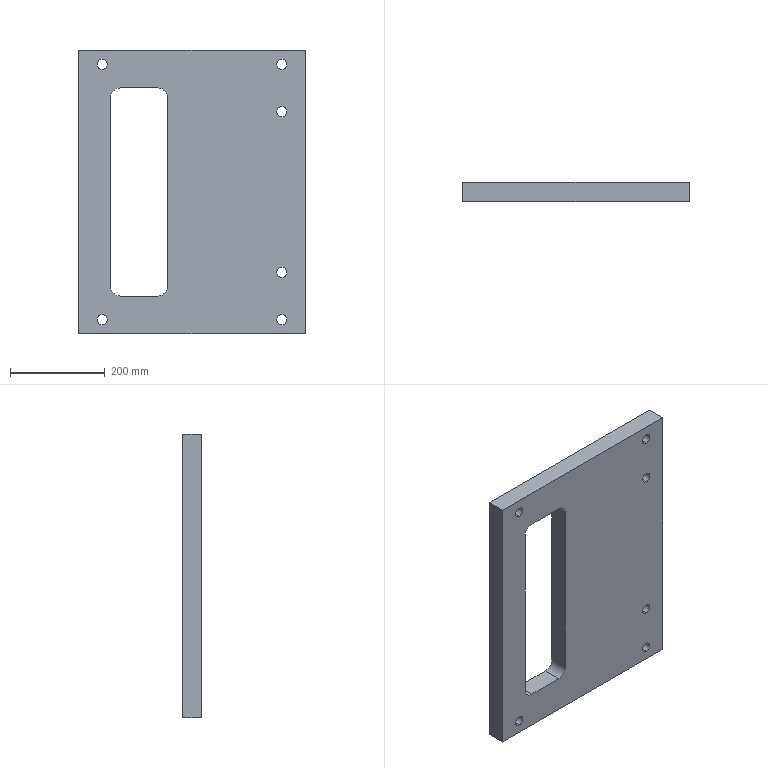Part | SolidWorks | features Extrusion 1, Fillet 1, HoleWzd 1, ICE 1 | 1 solid | 26 faces | box 480 x 40 x 600 mm | volume 9338608 mm3 | cylinder 16 | plane 10 | commonest cylinder face diameters 21 x12 40 x4
STEP:
#1=CARTESIAN_POINT('',(-190.,0.,259.5));
#2=VERTEX_POINT('',#1);
#3=CARTESIAN_POINT('',(-190.,0.,280.5));
#4=VERTEX_POINT('',#3);
#5=CARTESIAN_POINT('',(-190.,0.,270.));
#6=DIRECTION('',(0.,1.,0.));
#7=DIRECTION('',(0.,0.,1.));
#8=AXIS2_PLACEMENT_3D('',#5,#6,#7);
#9=CIRCLE('',#8,10.5);
#10=EDGE_CURVE('',#2,#4,#9,.T.);
#11=ORIENTED_EDGE('',*,*,#10,.F.);
#12=CARTESIAN_POINT('',(-190.,40.,259.5));
#13=VERTEX_POINT('',#12);
#14=CARTESIAN_POINT('',(-190.,40.,259.5));
#15=DIRECTION('',(0.,1.,0.));
#16=VECTOR('',#15,1000.);
#17=LINE('',#14,#16);
#18=EDGE_CURVE('',#2,#13,#17,.T.);
#19=ORIENTED_EDGE('',*,*,#18,.T.);
#20=CARTESIAN_POINT('',(-190.,40.,280.5));
#21=VERTEX_POINT('',#20);
#22=CARTESIAN_POINT('',(-190.,40.,270.));
#23=DIRECTION('',(0.,1.,0.));
#24=DIRECTION('',(0.,0.,1.));
#25=AXIS2_PLACEMENT_3D('',#22,#23,#24);
#26=CIRCLE('',#25,10.5);
#27=EDGE_CURVE('',#13,#21,#26,.T.);
#28=ORIENTED_EDGE('',*,*,#27,.T.);
#29=CARTESIAN_POINT('',(-190.,40.,280.5));
#30=DIRECTION('',(0.,1.,0.));
#31=VECTOR('',#30,1000.);
#32=LINE('',#29,#31);
#33=EDGE_CURVE('',#4,#21,#32,.T.);
#34=ORIENTED_EDGE('',*,*,#33,.F.);
#35=EDGE_LOOP('',(#11,#19,#28,#34));
#36=FACE_OUTER_BOUND('',#35,.T.);
#37=CARTESIAN_POINT('',(-190.,40.,270.));
#38=DIRECTION('',(0.,1.,0.));
#39=DIRECTION('',(0.,0.,1.));
#40=AXIS2_PLACEMENT_3D('',#37,#38,#39);
#41=CYLINDRICAL_SURFACE('',#40,10.5);
#42=ADVANCED_FACE('',(#36),#41,.F.);
#43=CARTESIAN_POINT('',(-190.,0.,-280.5));
#44=VERTEX_POINT('',#43);
#45=CARTESIAN_POINT('',(-190.,0.,-259.5));
#46=VERTEX_POINT('',#45);
#47=CARTESIAN_POINT('',(-190.,0.,-270.));
#48=DIRECTION('',(0.,1.,0.));
#49=DIRECTION('',(0.,0.,1.));
#50=AXIS2_PLACEMENT_3D('',#47,#48,#49);
#51=CIRCLE('',#50,10.5);
#52=EDGE_CURVE('',#44,#46,#51,.T.);
#53=ORIENTED_EDGE('',*,*,#52,.F.);
#54=CARTESIAN_POINT('',(-190.,40.,-280.5));
#55=VERTEX_POINT('',#54);
#56=CARTESIAN_POINT('',(-190.,40.,-280.5));
#57=DIRECTION('',(0.,1.,0.));
#58=VECTOR('',#57,1000.);
#59=LINE('',#56,#58);
#60=EDGE_CURVE('',#44,#55,#59,.T.);
#61=ORIENTED_EDGE('',*,*,#60,.T.);
#62=CARTESIAN_POINT('',(-190.,40.,-259.5));
#63=VERTEX_POINT('',#62);
#64=CARTESIAN_POINT('',(-190.,40.,-270.));
#65=DIRECTION('',(0.,1.,0.));
#66=DIRECTION('',(0.,0.,1.));
#67=AXIS2_PLACEMENT_3D('',#64,#65,#66);
#68=CIRCLE('',#67,10.5);
#69=EDGE_CURVE('',#55,#63,#68,.T.);
#70=ORIENTED_EDGE('',*,*,#69,.T.);
#71=CARTESIAN_POINT('',(-190.,40.,-259.5));
#72=DIRECTION('',(0.,1.,0.));
#73=VECTOR('',#72,1000.);
#74=LINE('',#71,#73);
#75=EDGE_CURVE('',#46,#63,#74,.T.);
#76=ORIENTED_EDGE('',*,*,#75,.F.);
#77=EDGE_LOOP('',(#53,#61,#70,#76));
#78=FACE_OUTER_BOUND('',#77,.T.);
#79=CARTESIAN_POINT('',(-190.,40.,-270.));
#80=DIRECTION('',(0.,1.,0.));
#81=DIRECTION('',(0.,0.,1.));
#82=AXIS2_PLACEMENT_3D('',#79,#80,#81);
#83=CYLINDRICAL_SURFACE('',#82,10.5);
#84=ADVANCED_FACE('',(#78),#83,.F.);
#85=CARTESIAN_POINT('',(190.,0.,-280.5));
#86=VERTEX_POINT('',#85);
#87=CARTESIAN_POINT('',(190.,0.,-259.5));
#88=VERTEX_POINT('',#87);
#89=CARTESIAN_POINT('',(190.,0.,-270.));
#90=DIRECTION('',(0.,1.,0.));
#91=DIRECTION('',(0.,0.,1.));
#92=AXIS2_PLACEMENT_3D('',#89,#90,#91);
#93=CIRCLE('',#92,10.5);
#94=EDGE_CURVE('',#86,#88,#93,.T.);
#95=ORIENTED_EDGE('',*,*,#94,.F.);
#96=CARTESIAN_POINT('',(190.,40.,-280.5));
#97=VERTEX_POINT('',#96);
#98=CARTESIAN_POINT('',(190.,40.,-280.5));
#99=DIRECTION('',(0.,1.,0.));
#100=VECTOR('',#99,1000.);
#101=LINE('',#98,#100);
#102=EDGE_CURVE('',#86,#97,#101,.T.);
#103=ORIENTED_EDGE('',*,*,#102,.T.);
#104=CARTESIAN_POINT('',(190.,40.,-259.5));
#105=VERTEX_POINT('',#104);
#106=CARTESIAN_POINT('',(190.,40.,-270.));
#107=DIRECTION('',(0.,1.,0.));
#108=DIRECTION('',(0.,0.,1.));
#109=AXIS2_PLACEMENT_3D('',#106,#107,#108);
#110=CIRCLE('',#109,10.5);
#111=EDGE_CURVE('',#97,#105,#110,.T.);
#112=ORIENTED_EDGE('',*,*,#111,.T.);
#113=CARTESIAN_POINT('',(190.,40.,-259.5));
#114=DIRECTION('',(0.,1.,0.));
#115=VECTOR('',#114,1000.);
#116=LINE('',#113,#115);
#117=EDGE_CURVE('',#88,#105,#116,.T.);
#118=ORIENTED_EDGE('',*,*,#117,.F.);
#119=EDGE_LOOP('',(#95,#103,#112,#118));
#120=FACE_OUTER_BOUND('',#119,.T.);
#121=CARTESIAN_POINT('',(190.,40.,-270.));
#122=DIRECTION('',(0.,1.,0.));
#123=DIRECTION('',(0.,0.,1.));
#124=AXIS2_PLACEMENT_3D('',#121,#122,#123);
#125=CYLINDRICAL_SURFACE('',#124,10.5);
#126=ADVANCED_FACE('',(#120),#125,.F.);
#127=CARTESIAN_POINT('',(190.,0.,259.5));
#128=VERTEX_POINT('',#127);
#129=CARTESIAN_POINT('',(190.,0.,280.5));
#130=VERTEX_POINT('',#129);
#131=CARTESIAN_POINT('',(190.,0.,270.));
#132=DIRECTION('',(0.,1.,0.));
#133=DIRECTION('',(0.,0.,1.));
#134=AXIS2_PLACEMENT_3D('',#131,#132,#133);
#135=CIRCLE('',#134,10.5);
#136=EDGE_CURVE('',#128,#130,#135,.T.);
#137=ORIENTED_EDGE('',*,*,#136,.F.);
#138=CARTESIAN_POINT('',(190.,40.,259.5));
#139=VERTEX_POINT('',#138);
#140=CARTESIAN_POINT('',(190.,40.,259.5));
#141=DIRECTION('',(0.,1.,0.));
#142=VECTOR('',#141,1000.);
#143=LINE('',#140,#142);
#144=EDGE_CURVE('',#128,#139,#143,.T.);
#145=ORIENTED_EDGE('',*,*,#144,.T.);
#146=CARTESIAN_POINT('',(190.,40.,280.5));
#147=VERTEX_POINT('',#146);
#148=CARTESIAN_POINT('',(190.,40.,270.));
#149=DIRECTION('',(0.,1.,0.));
#150=DIRECTION('',(0.,0.,1.));
#151=AXIS2_PLACEMENT_3D('',#148,#149,#150);
#152=CIRCLE('',#151,10.5);
#153=EDGE_CURVE('',#139,#147,#152,.T.);
#154=ORIENTED_EDGE('',*,*,#153,.T.);
#155=CARTESIAN_POINT('',(190.,40.,280.5));
#156=DIRECTION('',(0.,1.,0.));
#157=VECTOR('',#156,1000.);
#158=LINE('',#155,#157);
#159=EDGE_CURVE('',#130,#147,#158,.T.);
#160=ORIENTED_EDGE('',*,*,#159,.F.);
#161=EDGE_LOOP('',(#137,#145,#154,#160));
#162=FACE_OUTER_BOUND('',#161,.T.);
#163=CARTESIAN_POINT('',(190.,40.,270.));
#164=DIRECTION('',(0.,1.,0.));
#165=DIRECTION('',(0.,0.,1.));
#166=AXIS2_PLACEMENT_3D('',#163,#164,#165);
#167=CYLINDRICAL_SURFACE('',#166,10.5);
#168=ADVANCED_FACE('',(#162),#167,.F.);
#169=CARTESIAN_POINT('',(190.,0.,-180.5));
#170=VERTEX_POINT('',#169);
#171=CARTESIAN_POINT('',(190.,0.,-159.5));
#172=VERTEX_POINT('',#171);
#173=CARTESIAN_POINT('',(190.,0.,-170.));
#174=DIRECTION('',(0.,1.,0.));
#175=DIRECTION('',(0.,0.,1.));
#176=AXIS2_PLACEMENT_3D('',#173,#174,#175);
#177=CIRCLE('',#176,10.5);
#178=EDGE_CURVE('',#170,#172,#177,.T.);
#179=ORIENTED_EDGE('',*,*,#178,.F.);
#180=CARTESIAN_POINT('',(190.,40.,-180.5));
#181=VERTEX_POINT('',#180);
#182=CARTESIAN_POINT('',(190.,40.,-180.5));
#183=DIRECTION('',(0.,1.,0.));
#184=VECTOR('',#183,1000.);
#185=LINE('',#182,#184);
#186=EDGE_CURVE('',#170,#181,#185,.T.);
#187=ORIENTED_EDGE('',*,*,#186,.T.);
#188=CARTESIAN_POINT('',(190.,40.,-159.5));
#189=VERTEX_POINT('',#188);
#190=CARTESIAN_POINT('',(190.,40.,-170.));
#191=DIRECTION('',(0.,1.,0.));
#192=DIRECTION('',(0.,0.,1.));
#193=AXIS2_PLACEMENT_3D('',#190,#191,#192);
#194=CIRCLE('',#193,10.5);
#195=EDGE_CURVE('',#181,#189,#194,.T.);
#196=ORIENTED_EDGE('',*,*,#195,.T.);
#197=CARTESIAN_POINT('',(190.,40.,-159.5));
#198=DIRECTION('',(0.,1.,0.));
#199=VECTOR('',#198,1000.);
#200=LINE('',#197,#199);
#201=EDGE_CURVE('',#172,#189,#200,.T.);
#202=ORIENTED_EDGE('',*,*,#201,.F.);
#203=EDGE_LOOP('',(#179,#187,#196,#202));
#204=FACE_OUTER_BOUND('',#203,.T.);
#205=CARTESIAN_POINT('',(190.,40.,-170.));
#206=DIRECTION('',(0.,1.,0.));
#207=DIRECTION('',(0.,0.,1.));
#208=AXIS2_PLACEMENT_3D('',#205,#206,#207);
#209=CYLINDRICAL_SURFACE('',#208,10.5);
#210=ADVANCED_FACE('',(#204),#209,.F.);
#211=CARTESIAN_POINT('',(190.,0.,159.5));
#212=VERTEX_POINT('',#211);
#213=CARTESIAN_POINT('',(190.,0.,180.5));
#214=VERTEX_POINT('',#213);
#215=CARTESIAN_POINT('',(190.,0.,170.));
#216=DIRECTION('',(0.,1.,0.));
#217=DIRECTION('',(0.,0.,1.));
#218=AXIS2_PLACEMENT_3D('',#215,#216,#217);
#219=CIRCLE('',#218,10.5);
#220=EDGE_CURVE('',#212,#214,#219,.T.);
#221=ORIENTED_EDGE('',*,*,#220,.F.);
#222=CARTESIAN_POINT('',(190.,40.,159.5));
#223=VERTEX_POINT('',#222);
#224=CARTESIAN_POINT('',(190.,40.,159.5));
#225=DIRECTION('',(0.,1.,0.));
#226=VECTOR('',#225,1000.);
#227=LINE('',#224,#226);
#228=EDGE_CURVE('',#212,#223,#227,.T.);
#229=ORIENTED_EDGE('',*,*,#228,.T.);
#230=CARTESIAN_POINT('',(190.,40.,180.5));
#231=VERTEX_POINT('',#230);
#232=CARTESIAN_POINT('',(190.,40.,170.));
#233=DIRECTION('',(0.,1.,0.));
#234=DIRECTION('',(0.,0.,1.));
#235=AXIS2_PLACEMENT_3D('',#232,#233,#234);
#236=CIRCLE('',#235,10.5);
#237=EDGE_CURVE('',#223,#231,#236,.T.);
#238=ORIENTED_EDGE('',*,*,#237,.T.);
#239=CARTESIAN_POINT('',(190.,40.,180.5));
#240=DIRECTION('',(0.,1.,0.));
#241=VECTOR('',#240,1000.);
#242=LINE('',#239,#241);
#243=EDGE_CURVE('',#214,#231,#242,.T.);
#244=ORIENTED_EDGE('',*,*,#243,.F.);
#245=EDGE_LOOP('',(#221,#229,#238,#244));
#246=FACE_OUTER_BOUND('',#245,.T.);
#247=CARTESIAN_POINT('',(190.,40.,170.));
#248=DIRECTION('',(0.,1.,0.));
#249=DIRECTION('',(0.,0.,1.));
#250=AXIS2_PLACEMENT_3D('',#247,#248,#249);
#251=CYLINDRICAL_SURFACE('',#250,10.5);
#252=ADVANCED_FACE('',(#246),#251,.F.);
#253=CARTESIAN_POINT('',(240.,0.,300.));
#254=VERTEX_POINT('',#253);
#255=CARTESIAN_POINT('',(240.,0.,-300.));
#256=VERTEX_POINT('',#255);
#257=CARTESIAN_POINT('',(240.,0.,-300.));
#258=DIRECTION('',(0.,0.,-1.));
#259=VECTOR('',#258,1000.);
#260=LINE('',#257,#259);
#261=EDGE_CURVE('',#254,#256,#260,.T.);
#262=ORIENTED_EDGE('',*,*,#261,.T.);
#263=CARTESIAN_POINT('',(240.,40.,-300.));
#264=VERTEX_POINT('',#263);
#265=CARTESIAN_POINT('',(240.,40.,-300.));
#266=DIRECTION('',(0.,-1.,0.));
#267=VECTOR('',#266,1000.);
#268=LINE('',#265,#267);
#269=EDGE_CURVE('',#264,#256,#268,.T.);
#270=ORIENTED_EDGE('',*,*,#269,.F.);
#271=CARTESIAN_POINT('',(240.,40.,300.));
#272=VERTEX_POINT('',#271);
#273=CARTESIAN_POINT('',(240.,40.,-300.));
#274=DIRECTION('',(0.,0.,-1.));
#275=VECTOR('',#274,1000.);
#276=LINE('',#273,#275);
#277=EDGE_CURVE('',#272,#264,#276,.T.);
#278=ORIENTED_EDGE('',*,*,#277,.F.);
#279=CARTESIAN_POINT('',(240.,40.,300.));
#280=DIRECTION('',(0.,-1.,0.));
#281=VECTOR('',#280,1000.);
#282=LINE('',#279,#281);
#283=EDGE_CURVE('',#272,#254,#282,.T.);
#284=ORIENTED_EDGE('',*,*,#283,.T.);
#285=EDGE_LOOP('',(#262,#270,#278,#284));
#286=FACE_OUTER_BOUND('',#285,.T.);
#287=CARTESIAN_POINT('',(240.,40.,-300.));
#288=DIRECTION('',(-1.,0.,0.));
#289=DIRECTION('',(0.,0.,1.));
#290=AXIS2_PLACEMENT_3D('',#287,#288,#289);
#291=PLANE('',#290);
#292=ADVANCED_FACE('',(#286),#291,.F.);
#293=CARTESIAN_POINT('',(-240.,0.,-300.));
#294=VERTEX_POINT('',#293);
#295=CARTESIAN_POINT('',(-240.,0.,-300.));
#296=DIRECTION('',(-1.,0.,0.));
#297=VECTOR('',#296,1000.);
#298=LINE('',#295,#297);
#299=EDGE_CURVE('',#256,#294,#298,.T.);
#300=ORIENTED_EDGE('',*,*,#299,.T.);
#301=CARTESIAN_POINT('',(-240.,40.,-300.));
#302=VERTEX_POINT('',#301);
#303=CARTESIAN_POINT('',(-240.,40.,-300.));
#304=DIRECTION('',(0.,-1.,0.));
#305=VECTOR('',#304,1000.);
#306=LINE('',#303,#305);
#307=EDGE_CURVE('',#302,#294,#306,.T.);
#308=ORIENTED_EDGE('',*,*,#307,.F.);
#309=CARTESIAN_POINT('',(-240.,40.,-300.));
#310=DIRECTION('',(-1.,0.,0.));
#311=VECTOR('',#310,1000.);
#312=LINE('',#309,#311);
#313=EDGE_CURVE('',#264,#302,#312,.T.);
#314=ORIENTED_EDGE('',*,*,#313,.F.);
#315=ORIENTED_EDGE('',*,*,#269,.T.);
#316=EDGE_LOOP('',(#300,#308,#314,#315));
#317=FACE_OUTER_BOUND('',#316,.T.);
#318=CARTESIAN_POINT('',(-240.,40.,-300.));
#319=DIRECTION('',(0.,0.,1.));
#320=DIRECTION('',(1.,0.,0.));
#321=AXIS2_PLACEMENT_3D('',#318,#319,#320);
#322=PLANE('',#321);
#323=ADVANCED_FACE('',(#317),#322,.F.);
#324=CARTESIAN_POINT('',(-240.,0.,300.));
#325=VERTEX_POINT('',#324);
#326=CARTESIAN_POINT('',(-240.,0.,-300.));
#327=DIRECTION('',(0.,0.,1.));
#328=VECTOR('',#327,1000.);
#329=LINE('',#326,#328);
#330=EDGE_CURVE('',#294,#325,#329,.T.);
#331=ORIENTED_EDGE('',*,*,#330,.T.);
#332=CARTESIAN_POINT('',(-240.,40.,300.));
#333=VERTEX_POINT('',#332);
#334=CARTESIAN_POINT('',(-240.,40.,300.));
#335=DIRECTION('',(0.,-1.,0.));
#336=VECTOR('',#335,1000.);
#337=LINE('',#334,#336);
#338=EDGE_CURVE('',#333,#325,#337,.T.);
#339=ORIENTED_EDGE('',*,*,#338,.F.);
#340=CARTESIAN_POINT('',(-240.,40.,-300.));
#341=DIRECTION('',(0.,0.,1.));
#342=VECTOR('',#341,1000.);
#343=LINE('',#340,#342);
#344=EDGE_CURVE('',#302,#333,#343,.T.);
#345=ORIENTED_EDGE('',*,*,#344,.F.);
#346=ORIENTED_EDGE('',*,*,#307,.T.);
#347=EDGE_LOOP('',(#331,#339,#345,#346));
#348=FACE_OUTER_BOUND('',#347,.T.);
#349=CARTESIAN_POINT('',(-240.,40.,-300.));
#350=DIRECTION('',(1.,0.,0.));
#351=DIRECTION('',(0.,0.,-1.));
#352=AXIS2_PLACEMENT_3D('',#349,#350,#351);
#353=PLANE('',#352);
#354=ADVANCED_FACE('',(#348),#353,.F.);
#355=CARTESIAN_POINT('',(-240.,0.,300.));
#356=DIRECTION('',(1.,0.,0.));
#357=VECTOR('',#356,1000.);
#358=LINE('',#355,#357);
#359=EDGE_CURVE('',#325,#254,#358,.T.);
#360=ORIENTED_EDGE('',*,*,#359,.T.);
#361=ORIENTED_EDGE('',*,*,#283,.F.);
#362=CARTESIAN_POINT('',(-240.,40.,300.));
#363=DIRECTION('',(1.,0.,0.));
#364=VECTOR('',#363,1000.);
#365=LINE('',#362,#364);
#366=EDGE_CURVE('',#333,#272,#365,.T.);
#367=ORIENTED_EDGE('',*,*,#366,.F.);
#368=ORIENTED_EDGE('',*,*,#338,.T.);
#369=EDGE_LOOP('',(#360,#361,#367,#368));
#370=FACE_OUTER_BOUND('',#369,.T.);
#371=CARTESIAN_POINT('',(-240.,40.,300.));
#372=DIRECTION('',(0.,0.,-1.));
#373=DIRECTION('',(-1.,0.,0.));
#374=AXIS2_PLACEMENT_3D('',#371,#372,#373);
#375=PLANE('',#374);
#376=ADVANCED_FACE('',(#370),#375,.F.);
#377=CARTESIAN_POINT('',(-190.,40.,270.));
#378=DIRECTION('',(0.,1.,0.));
#379=DIRECTION('',(0.,0.,1.));
#380=AXIS2_PLACEMENT_3D('',#377,#378,#379);
#381=CIRCLE('',#380,10.5);
#382=EDGE_CURVE('',#21,#13,#381,.T.);
#383=ORIENTED_EDGE('',*,*,#382,.F.);
#384=ORIENTED_EDGE('',*,*,#27,.F.);
#385=EDGE_LOOP('',(#383,#384));
#386=FACE_BOUND('',#385,.T.);
#387=CARTESIAN_POINT('',(-190.,40.,-270.));
#388=DIRECTION('',(0.,1.,0.));
#389=DIRECTION('',(0.,0.,1.));
#390=AXIS2_PLACEMENT_3D('',#387,#388,#389);
#391=CIRCLE('',#390,10.5);
#392=EDGE_CURVE('',#63,#55,#391,.T.);
#393=ORIENTED_EDGE('',*,*,#392,.F.);
#394=ORIENTED_EDGE('',*,*,#69,.F.);
#395=EDGE_LOOP('',(#393,#394));
#396=FACE_BOUND('',#395,.T.);
#397=CARTESIAN_POINT('',(190.,40.,-270.));
#398=DIRECTION('',(0.,1.,0.));
#399=DIRECTION('',(0.,0.,1.));
#400=AXIS2_PLACEMENT_3D('',#397,#398,#399);
#401=CIRCLE('',#400,10.5);
#402=EDGE_CURVE('',#105,#97,#401,.T.);
#403=ORIENTED_EDGE('',*,*,#402,.F.);
#404=ORIENTED_EDGE('',*,*,#111,.F.);
#405=EDGE_LOOP('',(#403,#404));
#406=FACE_BOUND('',#405,.T.);
#407=CARTESIAN_POINT('',(190.,40.,270.));
#408=DIRECTION('',(0.,1.,0.));
#409=DIRECTION('',(0.,0.,1.));
#410=AXIS2_PLACEMENT_3D('',#407,#408,#409);
#411=CIRCLE('',#410,10.5);
#412=EDGE_CURVE('',#147,#139,#411,.T.);
#413=ORIENTED_EDGE('',*,*,#412,.F.);
#414=ORIENTED_EDGE('',*,*,#153,.F.);
#415=EDGE_LOOP('',(#413,#414));
#416=FACE_BOUND('',#415,.T.);
#417=CARTESIAN_POINT('',(190.,40.,-170.));
#418=DIRECTION('',(0.,1.,0.));
#419=DIRECTION('',(0.,0.,1.));
#420=AXIS2_PLACEMENT_3D('',#417,#418,#419);
#421=CIRCLE('',#420,10.5);
#422=EDGE_CURVE('',#189,#181,#421,.T.);
#423=ORIENTED_EDGE('',*,*,#422,.F.);
#424=ORIENTED_EDGE('',*,*,#195,.F.);
#425=EDGE_LOOP('',(#423,#424));
#426=FACE_BOUND('',#425,.T.);
#427=CARTESIAN_POINT('',(190.,40.,170.));
#428=DIRECTION('',(0.,1.,0.));
#429=DIRECTION('',(0.,0.,1.));
#430=AXIS2_PLACEMENT_3D('',#427,#428,#429);
#431=CIRCLE('',#430,10.5);
#432=EDGE_CURVE('',#231,#223,#431,.T.);
#433=ORIENTED_EDGE('',*,*,#432,.F.);
#434=ORIENTED_EDGE('',*,*,#237,.F.);
#435=EDGE_LOOP('',(#433,#434));
#436=FACE_BOUND('',#435,.T.);
#437=CARTESIAN_POINT('',(-52.,40.,200.));
#438=VERTEX_POINT('',#437);
#439=CARTESIAN_POINT('',(-52.,40.,-200.));
#440=VERTEX_POINT('',#439);
#441=CARTESIAN_POINT('',(-52.,40.,-220.));
#442=DIRECTION('',(0.,0.,-1.));
#443=VECTOR('',#442,1000.);
#444=LINE('',#441,#443);
#445=EDGE_CURVE('',#438,#440,#444,.T.);
#446=ORIENTED_EDGE('',*,*,#445,.F.);
#447=CARTESIAN_POINT('',(-72.,40.,220.));
#448=VERTEX_POINT('',#447);
#449=CARTESIAN_POINT('',(-72.,40.,200.));
#450=DIRECTION('',(0.,-1.,0.));
#451=DIRECTION('',(0.,0.,1.));
#452=AXIS2_PLACEMENT_3D('',#449,#450,#451);
#453=CIRCLE('',#452,20.);
#454=EDGE_CURVE('',#438,#448,#453,.T.);
#455=ORIENTED_EDGE('',*,*,#454,.T.);
#456=CARTESIAN_POINT('',(-152.,40.,220.));
#457=VERTEX_POINT('',#456);
#458=CARTESIAN_POINT('',(-172.,40.,220.));
#459=DIRECTION('',(1.,0.,0.));
#460=VECTOR('',#459,1000.);
#461=LINE('',#458,#460);
#462=EDGE_CURVE('',#457,#448,#461,.T.);
#463=ORIENTED_EDGE('',*,*,#462,.F.);
#464=CARTESIAN_POINT('',(-172.,40.,200.));
#465=VERTEX_POINT('',#464);
#466=CARTESIAN_POINT('',(-152.,40.,200.));
#467=DIRECTION('',(0.,-1.,0.));
#468=DIRECTION('',(0.,0.,1.));
#469=AXIS2_PLACEMENT_3D('',#466,#467,#468);
#470=CIRCLE('',#469,20.);
#471=EDGE_CURVE('',#457,#465,#470,.T.);
#472=ORIENTED_EDGE('',*,*,#471,.T.);
#473=CARTESIAN_POINT('',(-172.,40.,-200.));
#474=VERTEX_POINT('',#473);
#475=CARTESIAN_POINT('',(-172.,40.,-220.));
#476=DIRECTION('',(0.,0.,1.));
#477=VECTOR('',#476,1000.);
#478=LINE('',#475,#477);
#479=EDGE_CURVE('',#474,#465,#478,.T.);
#480=ORIENTED_EDGE('',*,*,#479,.F.);
#481=CARTESIAN_POINT('',(-152.,40.,-220.));
#482=VERTEX_POINT('',#481);
#483=CARTESIAN_POINT('',(-152.,40.,-200.));
#484=DIRECTION('',(0.,-1.,0.));
#485=DIRECTION('',(0.,0.,1.));
#486=AXIS2_PLACEMENT_3D('',#483,#484,#485);
#487=CIRCLE('',#486,20.);
#488=EDGE_CURVE('',#474,#482,#487,.T.);
#489=ORIENTED_EDGE('',*,*,#488,.T.);
#490=CARTESIAN_POINT('',(-72.,40.,-220.));
#491=VERTEX_POINT('',#490);
#492=CARTESIAN_POINT('',(-172.,40.,-220.));
#493=DIRECTION('',(-1.,0.,0.));
#494=VECTOR('',#493,1000.);
#495=LINE('',#492,#494);
#496=EDGE_CURVE('',#491,#482,#495,.T.);
#497=ORIENTED_EDGE('',*,*,#496,.F.);
#498=CARTESIAN_POINT('',(-72.,40.,-200.));
#499=DIRECTION('',(0.,-1.,0.));
#500=DIRECTION('',(0.,0.,1.));
#501=AXIS2_PLACEMENT_3D('',#498,#499,#500);
#502=CIRCLE('',#501,20.);
#503=EDGE_CURVE('',#491,#440,#502,.T.);
#504=ORIENTED_EDGE('',*,*,#503,.T.);
#505=EDGE_LOOP('',(#446,#455,#463,#472,#480,#489,#497,#504));
#506=FACE_BOUND('',#505,.T.);
#507=ORIENTED_EDGE('',*,*,#277,.T.);
#508=ORIENTED_EDGE('',*,*,#313,.T.);
#509=ORIENTED_EDGE('',*,*,#344,.T.);
#510=ORIENTED_EDGE('',*,*,#366,.T.);
#511=EDGE_LOOP('',(#507,#508,#509,#510));
#512=FACE_OUTER_BOUND('',#511,.T.);
#513=CARTESIAN_POINT('',(0.,40.,0.));
#514=DIRECTION('',(0.,1.,0.));
#515=DIRECTION('',(0.,0.,1.));
#516=AXIS2_PLACEMENT_3D('',#513,#514,#515);
#517=PLANE('',#516);
#518=ADVANCED_FACE('',(#386,#396,#406,#416,#426,#436,#506,#512),#517,.T.);
#519=CARTESIAN_POINT('',(-190.,0.,270.));
#520=DIRECTION('',(0.,1.,0.));
#521=DIRECTION('',(0.,0.,1.));
#522=AXIS2_PLACEMENT_3D('',#519,#520,#521);
#523=CIRCLE('',#522,10.5);
#524=EDGE_CURVE('',#4,#2,#523,.T.);
#525=ORIENTED_EDGE('',*,*,#524,.T.);
#526=ORIENTED_EDGE('',*,*,#10,.T.);
#527=EDGE_LOOP('',(#525,#526));
#528=FACE_BOUND('',#527,.T.);
#529=CARTESIAN_POINT('',(-190.,0.,-270.));
#530=DIRECTION('',(0.,1.,0.));
#531=DIRECTION('',(0.,0.,1.));
#532=AXIS2_PLACEMENT_3D('',#529,#530,#531);
#533=CIRCLE('',#532,10.5);
#534=EDGE_CURVE('',#46,#44,#533,.T.);
#535=ORIENTED_EDGE('',*,*,#534,.T.);
#536=ORIENTED_EDGE('',*,*,#52,.T.);
#537=EDGE_LOOP('',(#535,#536));
#538=FACE_BOUND('',#537,.T.);
#539=CARTESIAN_POINT('',(190.,0.,-270.));
#540=DIRECTION('',(0.,1.,0.));
#541=DIRECTION('',(0.,0.,1.));
#542=AXIS2_PLACEMENT_3D('',#539,#540,#541);
#543=CIRCLE('',#542,10.5);
#544=EDGE_CURVE('',#88,#86,#543,.T.);
#545=ORIENTED_EDGE('',*,*,#544,.T.);
#546=ORIENTED_EDGE('',*,*,#94,.T.);
#547=EDGE_LOOP('',(#545,#546));
#548=FACE_BOUND('',#547,.T.);
#549=CARTESIAN_POINT('',(190.,0.,270.));
#550=DIRECTION('',(0.,1.,0.));
#551=DIRECTION('',(0.,0.,1.));
#552=AXIS2_PLACEMENT_3D('',#549,#550,#551);
#553=CIRCLE('',#552,10.5);
#554=EDGE_CURVE('',#130,#128,#553,.T.);
#555=ORIENTED_EDGE('',*,*,#554,.T.);
#556=ORIENTED_EDGE('',*,*,#136,.T.);
#557=EDGE_LOOP('',(#555,#556));
#558=FACE_BOUND('',#557,.T.);
#559=CARTESIAN_POINT('',(190.,0.,-170.));
#560=DIRECTION('',(0.,1.,0.));
#561=DIRECTION('',(0.,0.,1.));
#562=AXIS2_PLACEMENT_3D('',#559,#560,#561);
#563=CIRCLE('',#562,10.5);
#564=EDGE_CURVE('',#172,#170,#563,.T.);
#565=ORIENTED_EDGE('',*,*,#564,.T.);
#566=ORIENTED_EDGE('',*,*,#178,.T.);
#567=EDGE_LOOP('',(#565,#566));
#568=FACE_BOUND('',#567,.T.);
#569=CARTESIAN_POINT('',(190.,0.,170.));
#570=DIRECTION('',(0.,1.,0.));
#571=DIRECTION('',(0.,0.,1.));
#572=AXIS2_PLACEMENT_3D('',#569,#570,#571);
#573=CIRCLE('',#572,10.5);
#574=EDGE_CURVE('',#214,#212,#573,.T.);
#575=ORIENTED_EDGE('',*,*,#574,.T.);
#576=ORIENTED_EDGE('',*,*,#220,.T.);
#577=EDGE_LOOP('',(#575,#576));
#578=FACE_BOUND('',#577,.T.);
#579=CARTESIAN_POINT('',(-172.,0.,-200.));
#580=VERTEX_POINT('',#579);
#581=CARTESIAN_POINT('',(-172.,0.,200.));
#582=VERTEX_POINT('',#581);
#583=CARTESIAN_POINT('',(-172.,0.,-220.));
#584=DIRECTION('',(0.,0.,1.));
#585=VECTOR('',#584,1000.);
#586=LINE('',#583,#585);
#587=EDGE_CURVE('',#580,#582,#586,.T.);
#588=ORIENTED_EDGE('',*,*,#587,.T.);
#589=CARTESIAN_POINT('',(-152.,0.,220.));
#590=VERTEX_POINT('',#589);
#591=CARTESIAN_POINT('',(-152.,0.,200.));
#592=DIRECTION('',(0.,1.,0.));
#593=DIRECTION('',(0.,0.,1.));
#594=AXIS2_PLACEMENT_3D('',#591,#592,#593);
#595=CIRCLE('',#594,20.);
#596=EDGE_CURVE('',#582,#590,#595,.T.);
#597=ORIENTED_EDGE('',*,*,#596,.T.);
#598=CARTESIAN_POINT('',(-72.,0.,220.));
#599=VERTEX_POINT('',#598);
#600=CARTESIAN_POINT('',(-172.,0.,220.));
#601=DIRECTION('',(1.,0.,0.));
#602=VECTOR('',#601,1000.);
#603=LINE('',#600,#602);
#604=EDGE_CURVE('',#590,#599,#603,.T.);
#605=ORIENTED_EDGE('',*,*,#604,.T.);
#606=CARTESIAN_POINT('',(-52.,0.,200.));
#607=VERTEX_POINT('',#606);
#608=CARTESIAN_POINT('',(-72.,0.,200.));
#609=DIRECTION('',(0.,1.,0.));
#610=DIRECTION('',(0.,0.,1.));
#611=AXIS2_PLACEMENT_3D('',#608,#609,#610);
#612=CIRCLE('',#611,20.);
#613=EDGE_CURVE('',#599,#607,#612,.T.);
#614=ORIENTED_EDGE('',*,*,#613,.T.);
#615=CARTESIAN_POINT('',(-52.,0.,-200.));
#616=VERTEX_POINT('',#615);
#617=CARTESIAN_POINT('',(-52.,0.,-220.));
#618=DIRECTION('',(0.,0.,-1.));
#619=VECTOR('',#618,1000.);
#620=LINE('',#617,#619);
#621=EDGE_CURVE('',#607,#616,#620,.T.);
#622=ORIENTED_EDGE('',*,*,#621,.T.);
#623=CARTESIAN_POINT('',(-72.,0.,-220.));
#624=VERTEX_POINT('',#623);
#625=CARTESIAN_POINT('',(-72.,0.,-200.));
#626=DIRECTION('',(0.,1.,0.));
#627=DIRECTION('',(0.,0.,1.));
#628=AXIS2_PLACEMENT_3D('',#625,#626,#627);
#629=CIRCLE('',#628,20.);
#630=EDGE_CURVE('',#616,#624,#629,.T.);
#631=ORIENTED_EDGE('',*,*,#630,.T.);
#632=CARTESIAN_POINT('',(-152.,0.,-220.));
#633=VERTEX_POINT('',#632);
#634=CARTESIAN_POINT('',(-172.,0.,-220.));
#635=DIRECTION('',(-1.,0.,0.));
#636=VECTOR('',#635,1000.);
#637=LINE('',#634,#636);
#638=EDGE_CURVE('',#624,#633,#637,.T.);
#639=ORIENTED_EDGE('',*,*,#638,.T.);
#640=CARTESIAN_POINT('',(-152.,0.,-200.));
#641=DIRECTION('',(0.,1.,0.));
#642=DIRECTION('',(0.,0.,1.));
#643=AXIS2_PLACEMENT_3D('',#640,#641,#642);
#644=CIRCLE('',#643,20.);
#645=EDGE_CURVE('',#633,#580,#644,.T.);
#646=ORIENTED_EDGE('',*,*,#645,.T.);
#647=EDGE_LOOP('',(#588,#597,#605,#614,#622,#631,#639,#646));
#648=FACE_BOUND('',#647,.T.);
#649=ORIENTED_EDGE('',*,*,#261,.F.);
#650=ORIENTED_EDGE('',*,*,#359,.F.);
#651=ORIENTED_EDGE('',*,*,#330,.F.);
#652=ORIENTED_EDGE('',*,*,#299,.F.);
#653=EDGE_LOOP('',(#649,#650,#651,#652));
#654=FACE_OUTER_BOUND('',#653,.T.);
#655=CARTESIAN_POINT('',(0.,0.,0.));
#656=DIRECTION('',(0.,1.,0.));
#657=DIRECTION('',(0.,0.,1.));
#658=AXIS2_PLACEMENT_3D('',#655,#656,#657);
#659=PLANE('',#658);
#660=ADVANCED_FACE('',(#528,#538,#548,#558,#568,#578,#648,#654),#659,.F.);
#661=ORIENTED_EDGE('',*,*,#621,.F.);
#662=CARTESIAN_POINT('',(-52.,40.,200.));
#663=DIRECTION('',(0.,1.,0.));
#664=VECTOR('',#663,1000.);
#665=LINE('',#662,#664);
#666=EDGE_CURVE('',#607,#438,#665,.T.);
#667=ORIENTED_EDGE('',*,*,#666,.T.);
#668=ORIENTED_EDGE('',*,*,#445,.T.);
#669=CARTESIAN_POINT('',(-52.,0.,-200.));
#670=DIRECTION('',(0.,-1.,0.));
#671=VECTOR('',#670,1000.);
#672=LINE('',#669,#671);
#673=EDGE_CURVE('',#440,#616,#672,.T.);
#674=ORIENTED_EDGE('',*,*,#673,.T.);
#675=EDGE_LOOP('',(#661,#667,#668,#674));
#676=FACE_OUTER_BOUND('',#675,.T.);
#677=CARTESIAN_POINT('',(-52.,0.,-220.));
#678=DIRECTION('',(1.,0.,0.));
#679=DIRECTION('',(0.,0.,-1.));
#680=AXIS2_PLACEMENT_3D('',#677,#678,#679);
#681=PLANE('',#680);
#682=ADVANCED_FACE('',(#676),#681,.F.);
#683=ORIENTED_EDGE('',*,*,#462,.T.);
#684=CARTESIAN_POINT('',(-72.,0.,220.));
#685=DIRECTION('',(0.,-1.,0.));
#686=VECTOR('',#685,1000.);
#687=LINE('',#684,#686);
#688=EDGE_CURVE('',#448,#599,#687,.T.);
#689=ORIENTED_EDGE('',*,*,#688,.T.);
#690=ORIENTED_EDGE('',*,*,#604,.F.);
#691=CARTESIAN_POINT('',(-152.,40.,220.));
#692=DIRECTION('',(0.,1.,0.));
#693=VECTOR('',#692,1000.);
#694=LINE('',#691,#693);
#695=EDGE_CURVE('',#590,#457,#694,.T.);
#696=ORIENTED_EDGE('',*,*,#695,.T.);
#697=EDGE_LOOP('',(#683,#689,#690,#696));
#698=FACE_OUTER_BOUND('',#697,.T.);
#699=CARTESIAN_POINT('',(-172.,0.,220.));
#700=DIRECTION('',(0.,0.,1.));
#701=DIRECTION('',(1.,0.,0.));
#702=AXIS2_PLACEMENT_3D('',#699,#700,#701);
#703=PLANE('',#702);
#704=ADVANCED_FACE('',(#698),#703,.F.);
#705=ORIENTED_EDGE('',*,*,#479,.T.);
#706=CARTESIAN_POINT('',(-172.,0.,200.));
#707=DIRECTION('',(0.,-1.,0.));
#708=VECTOR('',#707,1000.);
#709=LINE('',#706,#708);
#710=EDGE_CURVE('',#465,#582,#709,.T.);
#711=ORIENTED_EDGE('',*,*,#710,.T.);
#712=ORIENTED_EDGE('',*,*,#587,.F.);
#713=CARTESIAN_POINT('',(-172.,40.,-200.));
#714=DIRECTION('',(0.,1.,0.));
#715=VECTOR('',#714,1000.);
#716=LINE('',#713,#715);
#717=EDGE_CURVE('',#580,#474,#716,.T.);
#718=ORIENTED_EDGE('',*,*,#717,.T.);
#719=EDGE_LOOP('',(#705,#711,#712,#718));
#720=FACE_OUTER_BOUND('',#719,.T.);
#721=CARTESIAN_POINT('',(-172.,0.,-220.));
#722=DIRECTION('',(-1.,0.,0.));
#723=DIRECTION('',(0.,0.,1.));
#724=AXIS2_PLACEMENT_3D('',#721,#722,#723);
#725=PLANE('',#724);
#726=ADVANCED_FACE('',(#720),#725,.F.);
#727=ORIENTED_EDGE('',*,*,#638,.F.);
#728=CARTESIAN_POINT('',(-72.,40.,-220.));
#729=DIRECTION('',(0.,1.,0.));
#730=VECTOR('',#729,1000.);
#731=LINE('',#728,#730);
#732=EDGE_CURVE('',#624,#491,#731,.T.);
#733=ORIENTED_EDGE('',*,*,#732,.T.);
#734=ORIENTED_EDGE('',*,*,#496,.T.);
#735=CARTESIAN_POINT('',(-152.,0.,-220.));
#736=DIRECTION('',(0.,-1.,0.));
#737=VECTOR('',#736,1000.);
#738=LINE('',#735,#737);
#739=EDGE_CURVE('',#482,#633,#738,.T.);
#740=ORIENTED_EDGE('',*,*,#739,.T.);
#741=EDGE_LOOP('',(#727,#733,#734,#740));
#742=FACE_OUTER_BOUND('',#741,.T.);
#743=CARTESIAN_POINT('',(-172.,0.,-220.));
#744=DIRECTION('',(0.,0.,-1.));
#745=DIRECTION('',(-1.,0.,0.));
#746=AXIS2_PLACEMENT_3D('',#743,#744,#745);
#747=PLANE('',#746);
#748=ADVANCED_FACE('',(#742),#747,.F.);
#749=ORIENTED_EDGE('',*,*,#613,.F.);
#750=ORIENTED_EDGE('',*,*,#688,.F.);
#751=ORIENTED_EDGE('',*,*,#454,.F.);
#752=ORIENTED_EDGE('',*,*,#666,.F.);
#753=EDGE_LOOP('',(#749,#750,#751,#752));
#754=FACE_OUTER_BOUND('',#753,.T.);
#755=CARTESIAN_POINT('',(-72.,0.,200.));
#756=DIRECTION('',(0.,-1.,0.));
#757=DIRECTION('',(0.,0.,-1.));
#758=AXIS2_PLACEMENT_3D('',#755,#756,#757);
#759=CYLINDRICAL_SURFACE('',#758,20.);
#760=ADVANCED_FACE('',(#754),#759,.F.);
#761=ORIENTED_EDGE('',*,*,#596,.F.);
#762=ORIENTED_EDGE('',*,*,#710,.F.);
#763=ORIENTED_EDGE('',*,*,#471,.F.);
#764=ORIENTED_EDGE('',*,*,#695,.F.);
#765=EDGE_LOOP('',(#761,#762,#763,#764));
#766=FACE_OUTER_BOUND('',#765,.T.);
#767=CARTESIAN_POINT('',(-152.,0.,200.));
#768=DIRECTION('',(0.,-1.,0.));
#769=DIRECTION('',(0.,0.,-1.));
#770=AXIS2_PLACEMENT_3D('',#767,#768,#769);
#771=CYLINDRICAL_SURFACE('',#770,20.);
#772=ADVANCED_FACE('',(#766),#771,.F.);
#773=ORIENTED_EDGE('',*,*,#630,.F.);
#774=ORIENTED_EDGE('',*,*,#673,.F.);
#775=ORIENTED_EDGE('',*,*,#503,.F.);
#776=ORIENTED_EDGE('',*,*,#732,.F.);
#777=EDGE_LOOP('',(#773,#774,#775,#776));
#778=FACE_OUTER_BOUND('',#777,.T.);
#779=CARTESIAN_POINT('',(-72.,0.,-200.));
#780=DIRECTION('',(0.,-1.,0.));
#781=DIRECTION('',(0.,0.,-1.));
#782=AXIS2_PLACEMENT_3D('',#779,#780,#781);
#783=CYLINDRICAL_SURFACE('',#782,20.);
#784=ADVANCED_FACE('',(#778),#783,.F.);
#785=ORIENTED_EDGE('',*,*,#645,.F.);
#786=ORIENTED_EDGE('',*,*,#739,.F.);
#787=ORIENTED_EDGE('',*,*,#488,.F.);
#788=ORIENTED_EDGE('',*,*,#717,.F.);
#789=EDGE_LOOP('',(#785,#786,#787,#788));
#790=FACE_OUTER_BOUND('',#789,.T.);
#791=CARTESIAN_POINT('',(-152.,0.,-200.));
#792=DIRECTION('',(0.,-1.,0.));
#793=DIRECTION('',(0.,0.,-1.));
#794=AXIS2_PLACEMENT_3D('',#791,#792,#793);
#795=CYLINDRICAL_SURFACE('',#794,20.);
#796=ADVANCED_FACE('',(#790),#795,.F.);
#797=ORIENTED_EDGE('',*,*,#228,.F.);
#798=ORIENTED_EDGE('',*,*,#574,.F.);
#799=ORIENTED_EDGE('',*,*,#243,.T.);
#800=ORIENTED_EDGE('',*,*,#432,.T.);
#801=EDGE_LOOP('',(#797,#798,#799,#800));
#802=FACE_OUTER_BOUND('',#801,.T.);
#803=CARTESIAN_POINT('',(190.,40.,170.));
#804=DIRECTION('',(0.,1.,0.));
#805=DIRECTION('',(0.,0.,1.));
#806=AXIS2_PLACEMENT_3D('',#803,#804,#805);
#807=CYLINDRICAL_SURFACE('',#806,10.5);
#808=ADVANCED_FACE('',(#802),#807,.F.);
#809=ORIENTED_EDGE('',*,*,#186,.F.);
#810=ORIENTED_EDGE('',*,*,#564,.F.);
#811=ORIENTED_EDGE('',*,*,#201,.T.);
#812=ORIENTED_EDGE('',*,*,#422,.T.);
#813=EDGE_LOOP('',(#809,#810,#811,#812));
#814=FACE_OUTER_BOUND('',#813,.T.);
#815=CARTESIAN_POINT('',(190.,40.,-170.));
#816=DIRECTION('',(0.,1.,0.));
#817=DIRECTION('',(0.,0.,1.));
#818=AXIS2_PLACEMENT_3D('',#815,#816,#817);
#819=CYLINDRICAL_SURFACE('',#818,10.5);
#820=ADVANCED_FACE('',(#814),#819,.F.);
#821=ORIENTED_EDGE('',*,*,#144,.F.);
#822=ORIENTED_EDGE('',*,*,#554,.F.);
#823=ORIENTED_EDGE('',*,*,#159,.T.);
#824=ORIENTED_EDGE('',*,*,#412,.T.);
#825=EDGE_LOOP('',(#821,#822,#823,#824));
#826=FACE_OUTER_BOUND('',#825,.T.);
#827=CARTESIAN_POINT('',(190.,40.,270.));
#828=DIRECTION('',(0.,1.,0.));
#829=DIRECTION('',(0.,0.,1.));
#830=AXIS2_PLACEMENT_3D('',#827,#828,#829);
#831=CYLINDRICAL_SURFACE('',#830,10.5);
#832=ADVANCED_FACE('',(#826),#831,.F.);
#833=ORIENTED_EDGE('',*,*,#102,.F.);
#834=ORIENTED_EDGE('',*,*,#544,.F.);
#835=ORIENTED_EDGE('',*,*,#117,.T.);
#836=ORIENTED_EDGE('',*,*,#402,.T.);
#837=EDGE_LOOP('',(#833,#834,#835,#836));
#838=FACE_OUTER_BOUND('',#837,.T.);
#839=CARTESIAN_POINT('',(190.,40.,-270.));
#840=DIRECTION('',(0.,1.,0.));
#841=DIRECTION('',(0.,0.,1.));
#842=AXIS2_PLACEMENT_3D('',#839,#840,#841);
#843=CYLINDRICAL_SURFACE('',#842,10.5);
#844=ADVANCED_FACE('',(#838),#843,.F.);
#845=ORIENTED_EDGE('',*,*,#60,.F.);
#846=ORIENTED_EDGE('',*,*,#534,.F.);
#847=ORIENTED_EDGE('',*,*,#75,.T.);
#848=ORIENTED_EDGE('',*,*,#392,.T.);
#849=EDGE_LOOP('',(#845,#846,#847,#848));
#850=FACE_OUTER_BOUND('',#849,.T.);
#851=CARTESIAN_POINT('',(-190.,40.,-270.));
#852=DIRECTION('',(0.,1.,0.));
#853=DIRECTION('',(0.,0.,1.));
#854=AXIS2_PLACEMENT_3D('',#851,#852,#853);
#855=CYLINDRICAL_SURFACE('',#854,10.5);
#856=ADVANCED_FACE('',(#850),#855,.F.);
#857=ORIENTED_EDGE('',*,*,#18,.F.);
#858=ORIENTED_EDGE('',*,*,#524,.F.);
#859=ORIENTED_EDGE('',*,*,#33,.T.);
#860=ORIENTED_EDGE('',*,*,#382,.T.);
#861=EDGE_LOOP('',(#857,#858,#859,#860));
#862=FACE_OUTER_BOUND('',#861,.T.);
#863=CARTESIAN_POINT('',(-190.,40.,270.));
#864=DIRECTION('',(0.,1.,0.));
#865=DIRECTION('',(0.,0.,1.));
#866=AXIS2_PLACEMENT_3D('',#863,#864,#865);
#867=CYLINDRICAL_SURFACE('',#866,10.5);
#868=ADVANCED_FACE('',(#862),#867,.F.);
#869=CLOSED_SHELL('',(#42,#84,#126,#168,#210,#252,#292,#323,#354,#376,#518,#660,#682,#704,#726,#748,#760,#772,#784,#796,#808,#820,#832,#844,#856,#868));
#870=MANIFOLD_SOLID_BREP('',#869);
#871=CARTESIAN_POINT('',(0.,0.,0.));
#872=DIRECTION('',(0.,0.,1.));
#873=DIRECTION('',(1.,0.,0.));
#874=AXIS2_PLACEMENT_3D('',#871,#872,#873);
#875=(LENGTH_UNIT()NAMED_UNIT(*)SI_UNIT(.MILLI.,.METRE.));
#876=UNCERTAINTY_MEASURE_WITH_UNIT(LENGTH_MEASURE(0.00001),#875,'','');
#877=(NAMED_UNIT(*)PLANE_ANGLE_UNIT()SI_UNIT($,.RADIAN.));
#878=(NAMED_UNIT(*)SI_UNIT($,.STERADIAN.)SOLID_ANGLE_UNIT());
#879=(GEOMETRIC_REPRESENTATION_CONTEXT(3)GLOBAL_UNCERTAINTY_ASSIGNED_CONTEXT((#876))GLOBAL_UNIT_ASSIGNED_CONTEXT((#875,#877,#878))REPRESENTATION_CONTEXT('',''));
#880=ADVANCED_BREP_SHAPE_REPRESENTATION('',(#870,#874),#879);